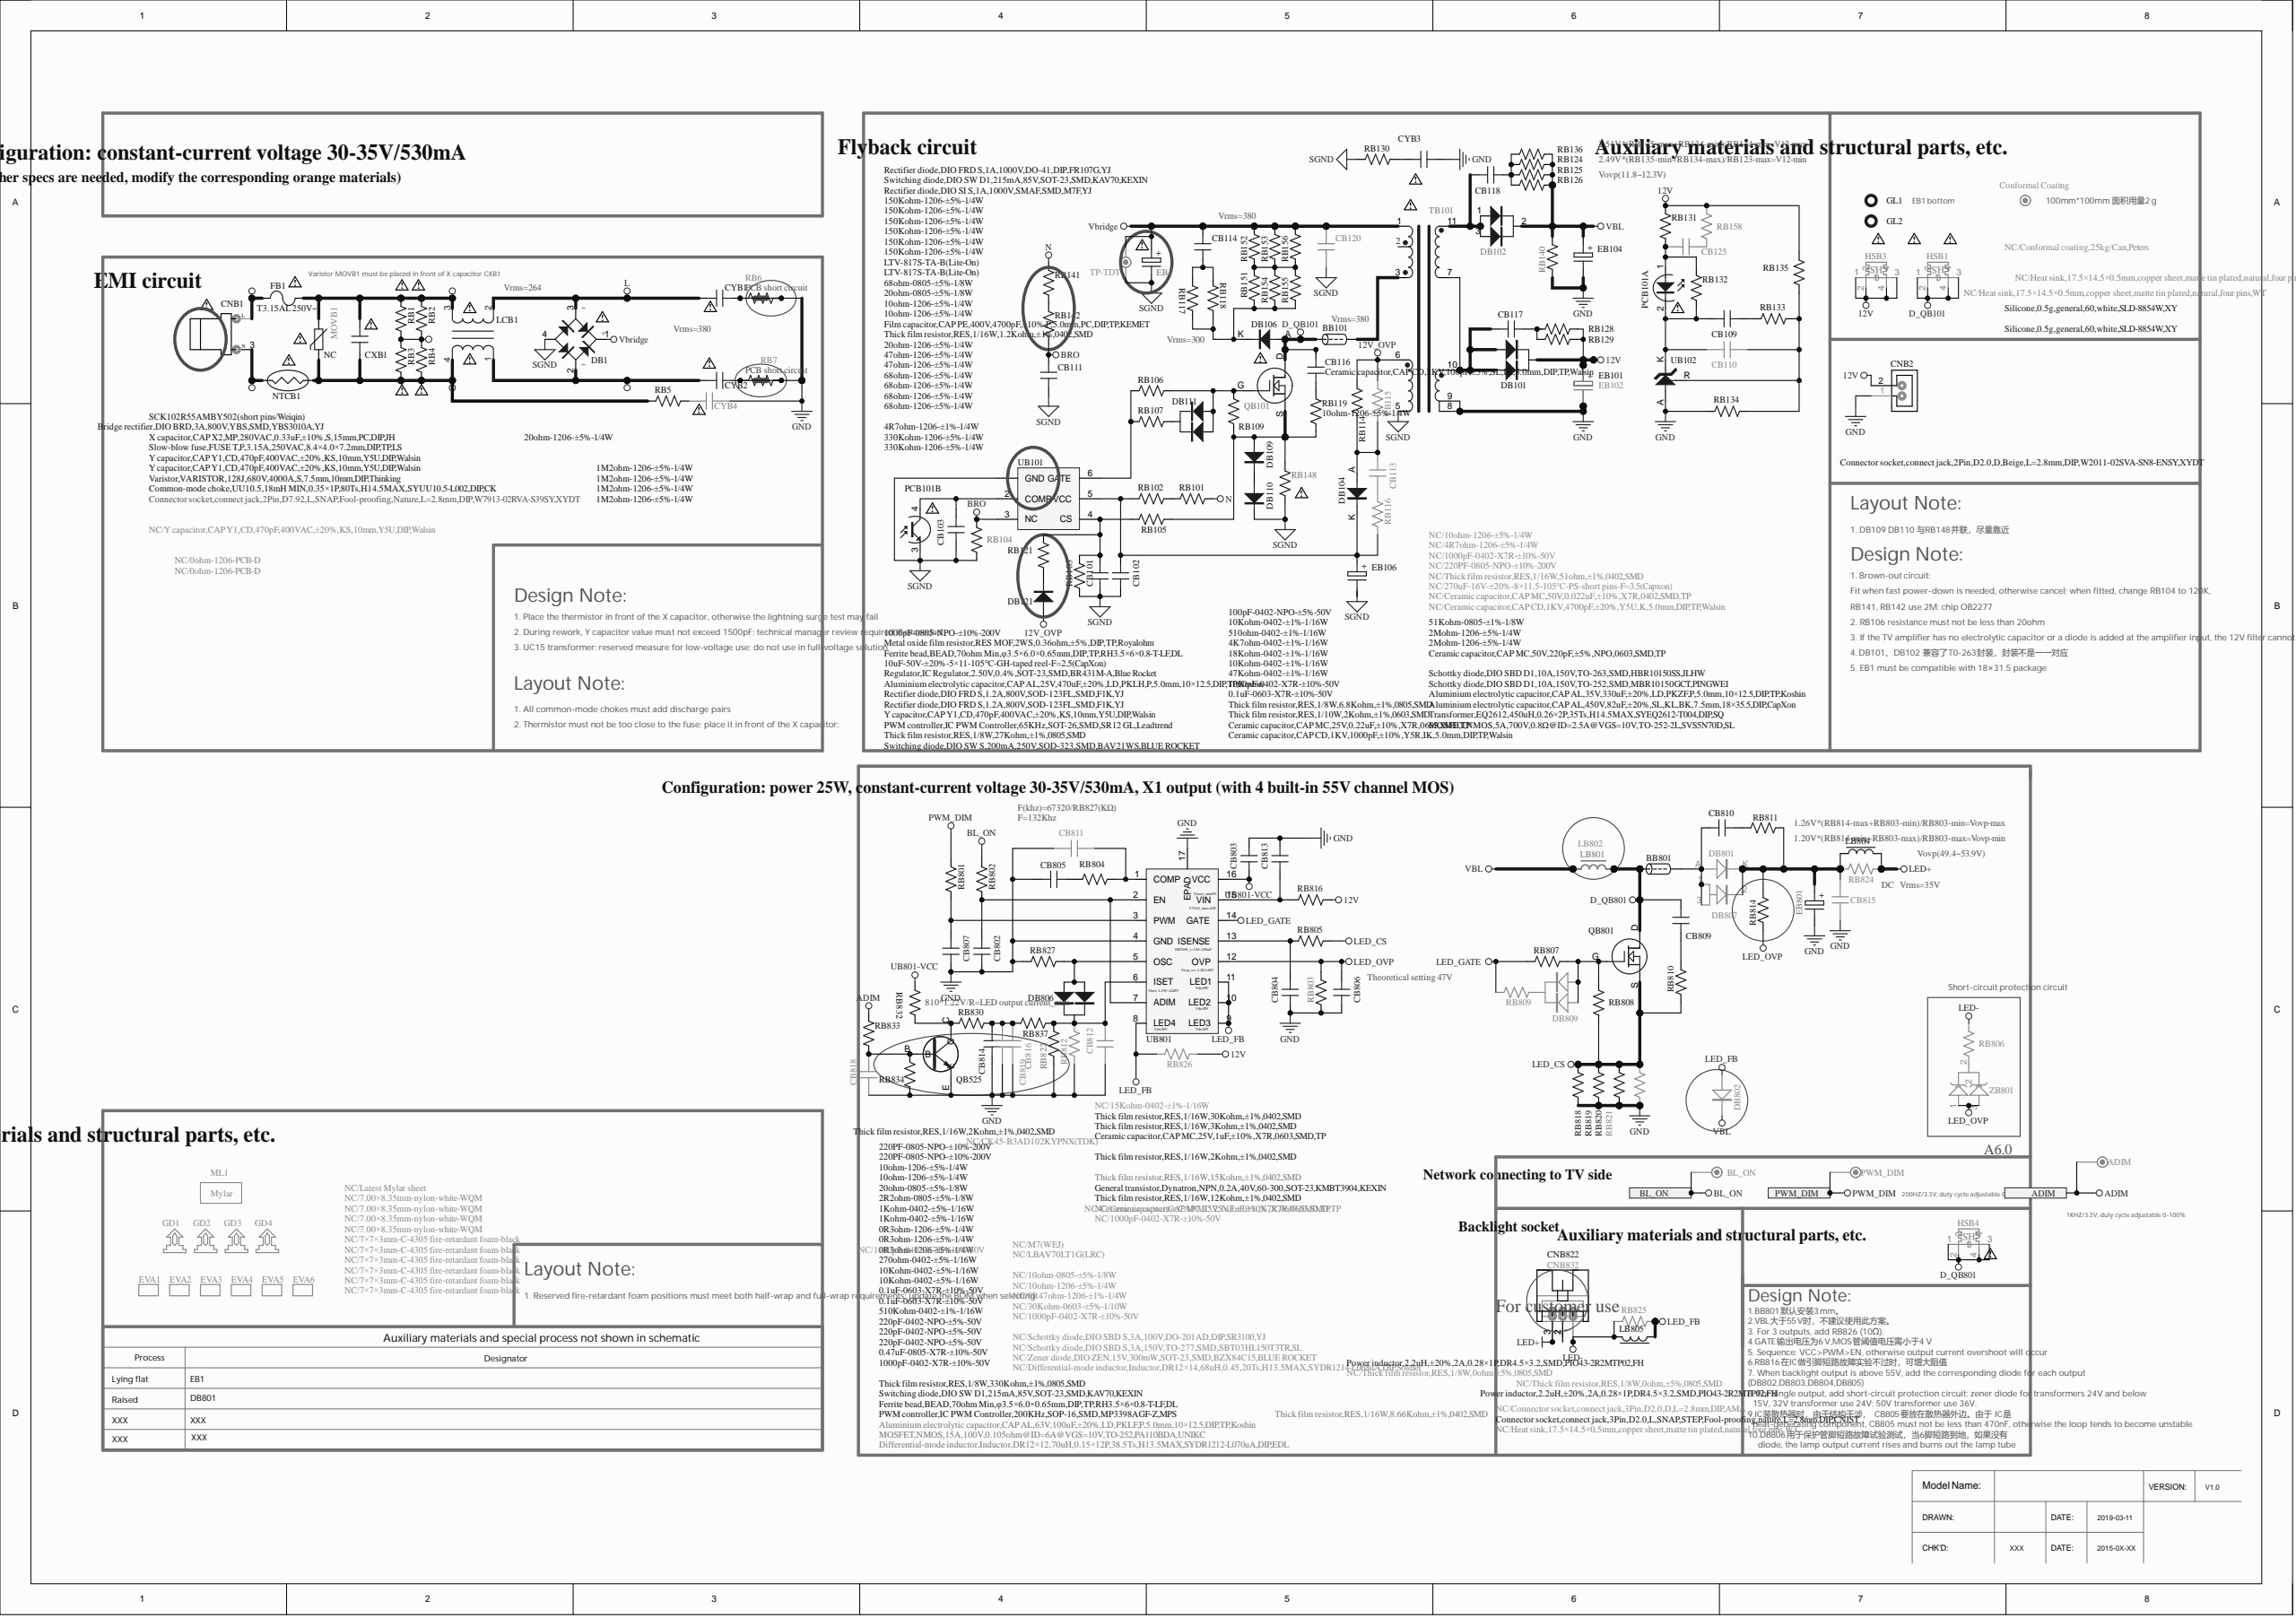Circuit board | Altium Designer | 951 parts | 509 nets | one sheet of the schematic
Parts on this sheet (reference | value | footprint):
BB101 | Ferrite bead,BEAD,70ohm Min,f3.5×6.0×0.65mm,DIP,TP,RH3.5×6×0.8-T-LF,DL | LB/3.5*6*12.5
BB801 | Ferrite bead,BEAD,70ohm Min,f3.5×6.0×0.65mm,DIP,TP,RH3.5×6×0.8-T-LF,DL | LB/3.5*6*12.5
CB101 | 100pF-0402-NPO-±5%-50V | C0402
CB102 | 0.1uF-0603-X7R-±10%-50V | C0603
CB103 | 1000pF-0402-X7R-±10%-50V | C0402
CB109 | Ceramic capacitor,CAP MC,25V,0.22uF,±10%,X7R,0603,SMD,TP | C0603
CB110 | NC/1000pF-0402-X7R-±10%-50V | C0402
CB111 | Ceramic capacitor,CAP MC,50V,220pF,±5%,NPO,0603,SMD,TP | C0603
CB113 | NC/220PF-0805-NPO-±10%-200V | C0805
CB114 | Film capacitor,CAP PE,400V,4700pF,±10%,P,5.0mm,PC,DIP,TP,KEMET | CAP8*2.5-V-5
CB116 | Ceramic capacitor,CAP CD,2KV,100pF,±5%,SL,IK,5.0mm,DIP,TP,Walsin | CAP6.5*5-V-5-1
CB117 | 1000pF-0805-NPO-±10%-200V | C0805
CB118 | Ceramic capacitor,CAP CD,1KV,1000pF,±10%,Y5R,IK,5.0mm,DIP,TP,Walsin | CAP8.5*5-V-5
CB120 | NC/Ceramic capacitor,CAP CD,1KV,4700pF,±20%,Y5U,K,5.0mm,DIP,TP,Walsin | CAP10*4.5-V-5
CB125 | NC/Ceramic capacitor,CAP MC,50V,0.022uF,±10%,X7R,0402,SMD,TP | C0402
CB802 | 220pF-0402-NPO-±5%-50V | C0402
CB803 | 0.1uF-0603-X7R-±10%-50V | C0603
CB804 | 220pF-0402-NPO-±5%-50V | C0402
CB805 | 0.47uF-0805-X7R-±10%-50V | C0805
CB806 | 1000pF-0402-X7R-±10%-50V | C0402
CB807 | 220pF-0402-NPO-±5%-50V | C0402
CB809 | 220PF-0805-NPO-±10%-200V | C0805
CB810 | 220PF-0805-NPO-±10%-200V | C0805
CB811 | NC/1000pF-0402-X7R-±10%-50V | C0402
CB812 | NC/1000pF-0402-X7R-±10%-50V | C0402
CB813 | 0.1uF-0603-X7R-±10%-50V | C0603
CB814 | Ceramic capacitor,CAP MC,25V,1uF,±10%,X7R,0603,SMD,TP | C0603
CB815 | NC/CK45-B3AD102KYPNX(TDK) | CAP7.5*2.5-V-5
CB816 | NC/Ceramic capacitor,CAP MC,25V,1uF,±10%,X7R,0603,SMD,TP | C0603
CB818 | NC/1000pF-0402-X7R-±10%-50V | C0402
CB819 | NC/Ceramic capacitor,CAP MC,25V,1uF,±10%,X7R,0603,SMD,TP | C0603
CNB1 | Connector socket,connect jack,2Pin,D7.92,L,SNAP,Fool-proofing,Nature,L=2.8mm,DIP,W7913-02RVA-S39SY,XYDT | CON2-H7.92
CNB2 | Connector socket,connect jack,2Pin,D2.0,D,Beige,L=2.8mm,DIP,W2011-02SVA-SN8-ENSY,XYDT | SIP2/2.0D-1
CNB822 | Connector socket,connect jack,3Pin,D2.0,L,SNAP,STEP,Fool-proofing,nature,L=2.8mm,DIP,CNJST | SIP3H/2.0D-3
CNB832 | NC/Connector socket,connect jack,3Pin,D2.0,D,L=2.8mm,DIP,AMA | SIP3/2.0D-CP
CXB1 | X capacitor,CAP X2,MP,280VAC,0.33uF,±10%,S,15mm,PC,DIP,JH | CAP18*8.5-V-15
CYB1 | Y capacitor,CAP Y1,CD,470pF,400VAC,±20%,KS,10mm,Y5U,DIP,Walsin | CAP13*5-V-10-1
CYB2 | Y capacitor,CAP Y1,CD,470pF,400VAC,±20%,KS,10mm,Y5U,DIP,Walsin | CAP13*5-V-10-1
CYB3 | Y capacitor,CAP Y1,CD,470pF,400VAC,±20%,KS,10mm,Y5U,DIP,Walsin | CAP13*5-V-10-1
CYB4 | NC/Y capacitor,CAP Y1,CD,470pF,400VAC,±20%,KS,10mm,Y5U,DIP,Walsin | CAP13*5-V-10-1
DB1 | Bridge rectifier,DIO BRD,3A,800V,YBS,SMD,YBS3010A,YJ | B/YBS3010A
DB101 | Schottky diode,DIO SBD D1,10A,150V,TO-252,SMD,MBR10150GCT,PINGWEI | D2PAK3
DB102 | Schottky diode,DIO SBD D1,10A,150V,TO-263,SMD,HBR10150SS,JLHW | D2PAK3
DB104 | Rectifier diode,DIO SI S,1A,1000V,SMAF,SMD,M7F,YJ | DIODE-S-2
DB106 | Rectifier diode,DIO FRD S,1A,1000V,DO-41,DIP,FR107G,YJ | D1-H-17.5
DB109 | Rectifier diode,DIO FRD S,1.2A,800V,SOD-123FL,SMD,F1K,YJ | DIODE-S-14
DB110 | Rectifier diode,DIO FRD S,1.2A,800V,SOD-123FL,SMD,F1K,YJ | DIODE-S-14
DB111 | Switching diode,DIO SW D1,215mA,85V,SOT-23,SMD,KAV70,KEXIN | SO-23
DB121 | Switching diode,DIO SW S,200mA,250V,SOD-323,SMD,BAV21WS,BLUE ROCKET | DIODE-S-12
DB801 | NC/Schottky diode,DIO SBD S,3A,100V,DO-201AD,DIP,SR3100,YJ | D3-H-20
DB802 | NC/M7(WEJ) | DIODE-S-2
DB806 | Switching diode,DIO SW D1,215mA,85V,SOT-23,SMD,KAV70,KEXIN | SO-23
DB807 | NC/Schottky diode,DIO SBD S,3A,150V,TO-277,SMD,SBT03HL150T3TR,SL | DIODE-S-13
DB809 | NC/LBAV70LT1G(LRC) | SO-23
EB1 | Aluminium electrolytic capacitor,CAP AL,450V,82uF,±20%,SL,KL,BK,7.5mm,18×35.5,DIP,CapXon | EC(18*41)-H-7.5-1
EB101 | Aluminium electrolytic capacitor,CAP AL,25V,470uF,±20%,LD,PKLH,P,5.0mm,10×12.5,DIP,TP,Koshin | EC(10*12.5)-V-5
EB102 | NC/270uF-16V-±20%-8×11.5-105℃-PS-short pins-F=3.5(Capxon) | EC(8*11)-V-3.5
EB104 | Aluminium electrolytic capacitor,CAP AL,35V,330uF,±20%,LD,PKZF,P,5.0mm,10×12.5,DIP,TP,Koshin | EC(10*12.5)-V-5
EB106 | 10uF-50V-±20%-5×11-105℃-GH-taped reel-F=2.5(CapXon) | EC(5*11)-V-2.5
EB801 | Aluminium electrolytic capacitor,CAP AL,63V,100uF,±20%,LD,PKLF,P,5.0mm,10×12.5,DIP,TP,Koshin | EC(10*12.5)-V-5
EVA1 | NC/7×7×3mm-C-4305 fire-retardant foam-black | EVA(7*7*3)
EVA2 | NC/7×7×3mm-C-4305 fire-retardant foam-black | EVA(7*7*3)
EVA3 | NC/7×7×3mm-C-4305 fire-retardant foam-black | EVA(7*7*3)
EVA4 | NC/7×7×3mm-C-4305 fire-retardant foam-black | EVA(7*7*3)
EVA5 | NC/7×7×3mm-C-4305 fire-retardant foam-black | EVA(7*7*3)
EVA6 | NC/7×7×3mm-C-4305 fire-retardant foam-black | EVA(7*7*3)
FB1 | Slow-blow fuse,FUSE T,P,3.15A,250VAC,8.4×4.0×7.2mm,DIP,TP,LS | FUSE8.5*4-V-5(T3.15AL 250V~)
GD1 | NC/7.00×8.35mm-nylon-white-WQM | Fixed
GD2 | NC/7.00×8.35mm-nylon-white-WQM | Fixed
GD3 | NC/7.00×8.35mm-nylon-white-WQM | Fixed
GD4 | NC/7.00×8.35mm-nylon-white-WQM | Fixed
GL1 | Silicone,0.5g,general,60,white,SLD-8854W,XY | Silica gel-15
GL2 | Silicone,0.5g,general,60,white,SLD-8854W,XY | Silica gel-10
HSB1 | NC/Heat sink,17.5×14.5×0.5mm,copper sheet,matte tin plated,natural,four pins,WT | HS149-YZ
HSB3 | NC/Heat sink,17.5×14.5×0.5mm,copper sheet,matte tin plated,natural,four pins,WT | HS149-YZ
HSB4 | NC/Heat sink,17.5×14.5×0.5mm,copper sheet,matte tin plated,natural,four pins,WT | HS149-YZ
LB801 | Differential-mode inductor,Inductor,DR12×12,70uH,0.15×12P,38.5Ts,H13.5MAX,SYDR1212-L070uA,DIP,EDL | L/LC2/15*14.5-V7.5
LB802 | NC/Differential-mode inductor,Inductor,DR12×14,68uH,0.45,20Ts,H13.5MAX,SYDR1214-L068uA,DIP,Soldier | L(13.5*15.5)-V-5
LB804 | Power inductor,2.2uH,±20%,2A,0.28×1P,DR4.5×3.2,SMD,PIO43-2R2MTP02,FH | L(4.5*3.5)-S
LB805 | Power inductor,2.2uH,±20%,2A,0.28×1P,DR4.5×3.2,SMD,PIO43-2R2MTP02,FH | L(4.5*3.5)-S
LCB1 | Common-mode choke,UU10.5,18mH MIN,0.35×1P,80Ts,H14.5MAX,SYUU10.5-L002,DIP,CK | L/UU10.5/10*13-2
ML1 | NC/Latest Mylar sheet | Mylar
MOVB1 | Varistor,VARISTOR,128J,680V,4000A,S,7.5mm,10mm,DIP,Thinking | VR(13*5)-V-7.5
NTCB1 | SCK102R55AMBY502(short pins/Weiqin) | NTC(10*5)-V5
PCB101 | LTV-817S-TA-B(Lite-On) | OC4-S-1
QB101 | MOSFET,NMOS,5A,700V,0.8Ω@ID=2.5A@VGS=10V,TO-252-2L,SVS5N70D,SL | TO-252-GDS
QB525 | General transistor,Dynatron,NPN,0.2A,40V,60-300,SOT-23,KMBT3904,KEXIN | SOT-23
QB801 | MOSFET,NMOS,15A,100V,0.105ohm@ID=6A@VGS=10V,TO-252,PA110BDA,UNIKC | TO-252-GDS
RB1 | 1M2ohm-1206-±5%-1/4W | R1206
RB2 | 1M2ohm-1206-±5%-1/4W | R1206
RB3 | 1M2ohm-1206-±5%-1/4W | R1206
RB4 | 1M2ohm-1206-±5%-1/4W | R1206
RB5 | 20ohm-1206-±5%-1/4W | R1206
RB6 | NC/0ohm-1206-PCB-D | R1206SC
RB7 | NC/0ohm-1206-PCB-D | R1206SC
RB101 | 330Kohm-1206-±5%-1/4W | R1206
RB102 | 330Kohm-1206-±5%-1/4W | R1206
RB103 | Thick film resistor,RES,1/8W,6.8Kohm,±1%,0805,SMD | R0402
RB104 | 47Kohm-0402-±1%-1/16W | R0402
RB105 | 510ohm-0402-±1%-1/16W | R0402
RB106 | 68ohm-0805-±5%-1/8W | R0805
RB107 | 20ohm-0805-±5%-1/8W | R0805
RB109 | 10Kohm-0402-±1%-1/16W | R0402
RB114 | 4R7ohm-1206-±1%-1/4W | R1206
RB115 | NC/4R7ohm-1206-±5%-1/4W | R1206
RB116 | NC/10ohm-1206-±5%-1/4W | R1206
RB117 | 10ohm-1206-±5%-1/4W | R1206
RB118 | 10ohm-1206-±5%-1/4W | R1206
RB119 | 10ohm-1206-±5%-1/4W | R1206
RB121 | Thick film resistor,RES,1/8W,27Kohm,±1%,0805,SMD | R0805
RB124 | 68ohm-1206-±5%-1/4W | R1206
RB125 | 68ohm-1206-±5%-1/4W | R1206
RB126 | 68ohm-1206-±5%-1/4W | R1206
RB128 | 47ohm-1206-±5%-1/4W | R1206
RB129 | 47ohm-1206-±5%-1/4W | R1206
RB130 | 20ohm-1206-±5%-1/4W | R1206
RB131 | Thick film resistor,RES,1/10W,2Kohm,±1%,0603,SMD | R0603
RB132 | Thick film resistor,RES,1/16W,1.2Kohm,±1%,0402,SMD | R0402
RB133 | 10Kohm-0402-±1%-1/16W | R0402
RB134 | 4K7ohm-0402-±1%-1/16W | R0402
RB135 | 18Kohm-0402-±1%-1/16W | R0402
RB136 | 68ohm-1206-±5%-1/4W | R1206
RB140 | 51Kohm-0805-±1%-1/8W | R0805
RB141 | 2Mohm-1206-±5%-1/4W | R1206
RB142 | 2Mohm-1206-±5%-1/4W | R1206
RB148 | Metal oxide film resistor,RES MOF,2WS,0.36ohm,±5%,DIP,TP,Royalohm | R2-H-17.5
RB151 | 150Kohm-1206-±5%-1/4W | R1206
RB152 | 150Kohm-1206-±5%-1/4W | R1206
RB153 | 150Kohm-1206-±5%-1/4W | R1206
RB154 | 150Kohm-1206-±5%-1/4W | R1206
RB155 | 150Kohm-1206-±5%-1/4W | R1206
RB156 | 150Kohm-1206-±5%-1/4W | R1206
RB158 | NC/Thick film resistor,RES,1/16W,51ohm,±1%,0402,SMD | R0402
RB801 | 1Kohm-0402-±5%-1/16W | R0402
RB802 | 10Kohm-0402-±5%-1/16W | R0402
RB803 | Thick film resistor,RES,1/16W,8.66Kohm,±1%,0402,SMD | R0402
RB804 | 270ohm-0402-±5%-1/16W | R0402
RB805 | 1Kohm-0402-±5%-1/16W | R0402
RB806 | NC/30Kohm-0603-±5%-1/10W | R0603
RB807 | 20ohm-0805-±5%-1/8W | R0805
RB808 | 10Kohm-0402-±5%-1/16W | R0402
RB809 | NC/10ohm-0805-±5%-1/8W | R0805
RB810 | 10ohm-1206-±5%-1/4W | R1206
RB811 | 10ohm-1206-±5%-1/4W | R1206
RB812 | NC/15Kohm-0402-±1%-1/16W | R0402
RB814 | Thick film resistor,RES,1/8W,330Kohm,±1%,0805,SMD | R0805
RB816 | 2R2ohm-0805-±5%-1/8W | R0805
RB818 | 0R3ohm-1206-±5%-1/4W | R1206
RB819 | 0R3ohm-1206-±5%-1/4W | R1206
RB820 | 0R3ohm-1206-±5%-1/4W | R1206
RB821 | NC/0R47ohm-1206-±1%-1/4W | R1206
RB822 | Thick film resistor,RES,1/16W,15Kohm,±1%,0402,SMD | R0402
RB824 | NC/Thick film resistor,RES,1/8W,0ohm,±5%,0805,SMD | R0805
RB825 | NC/Thick film resistor,RES,1/8W,0ohm,±5%,0805,SMD | R0805
RB826 | NC/10ohm-1206-±5%-1/4W | R1206
RB827 | 510Kohm-0402-±1%-1/16W | R0402
RB830 | Thick film resistor,RES,1/16W,3Kohm,±1%,0402,SMD | R0402
RB832 | Thick film resistor,RES,1/16W,30Kohm,±1%,0402,SMD | R0402
RB833 | Thick film resistor,RES,1/16W,2Kohm,±1%,0402,SMD | R0402
RB834 | Thick film resistor,RES,1/16W,2Kohm,±1%,0402,SMD | R0402
RB837 | Thick film resistor,RES,1/16W,12Kohm,±1%,0402,SMD | R0402
TB101 | Transformer,EQ2612,450uH,0.26×2P,35Ts,H14.5MAX,SYEQ2612-T004,DIP,SQ | T/EQ2512*11
TP-TDT | NC/ | TP-TDT
UB101 | PWM controller,IC PWM Controller,65KHz,SOT-26,SMD,SR12 GL,Leadtrend | SOT-26
UB102 | Regulator,IC Regulator,2.50V,0.4%,SOT-23,SMD,BR431M-A,Blue Rocket | SOT-23-RAK
UB801 | PWM controller,IC PWM Controller,200KHz,SOP-16,SMD,MP3398AGF-Z,MPS | TSSOP16/0.65-3
ZB801 | NC/Zener diode,DIO ZEN,15V,300mW,SOT-23,SMD,BZX84C15,BLUE ROCKET | SO-23
Nets of these parts (net: part-pin ...):
Vbridge: CB114-2 CB120-2 DB1-1 EB1-1 RB152-2 RB153-2 RB156-2 TB101-1 TP-TDT-1
VBL: DB102-2 DB802-K EB104-1 LB801-1 LB802-1 RB124-2 RB125-2 RB126-2 RB136-2 RB140-1
UB801-VCC: CB803-2 RB832-1 UB801-16
SGND: CB101-2 CB102-2 CB103-2 CB111-1 CB120-1 DB1-4 DB110-K EB1-2 EB106-2 PCB101-3 RB103-1 RB104-1 RB130-1 RB148-1 TB101-5 TP-TDT-2 UB101-1
PWM_DIM: RB801-1
NetRB806_2: RB806-2 ZB801-2
NetRB151_2: RB151-2 RB152-1 RB153-1 RB154-2 RB155-2 RB156-1
NetRB141_1: RB141-1 RB142-2
NetRB106_1: RB106-1 RB107-1 UB101-6
NetRB101_2: RB101-2 RB102-2
NetQB525_C: QB525-C RB830-2 RB832-2
NetDB809_2: DB809-2 RB809-2
NetDB809_1: DB809-1 DB809-3 QB801-G RB807-2 RB808-1
NetDB806_1: DB806-1 DB806-3 RB827-2 UB801-5
NetDB121_K: DB121-K RB121-1
NetDB111_2: DB111-2 RB107-2
NetDB111_1: DB111-1 DB111-3 QB101-G RB106-2 RB109-2
NetDB109_K: DB109-K DB110-A
NetDB109_A: DB109-A QB101-S RB105-2 RB109-1 RB119-1 RB148-2
NetDB106_K: DB106-K RB117-2 RB118-2 RB151-1 RB154-1 RB155-1
NetCYB4_1: CYB4-1 RB5-1
NetCYB3_1: CYB3-1 RB130-2
NetCNB822_2: CNB822-2 CNB832-2
NetCB818_2: CB818-2 QB525-B RB833-1 RB834-2
NetCB815_1: CB815-1 DB801-K DB807-2 EB801-1 LB804-1 RB811-2 RB814-2 RB824-1
NetCB814_1: CB814-1 CB816-1 CB819-1 RB830-1 RB837-1
NetCB813_2: CB813-2 RB816-1 UB801-15
NetCB812_2: CB812-2 DB806-2 RB812-2 RB822-2 RB837-2 UB801-6
NetCB811_1: CB811-1 RB804-2 UB801-1
NetCB810_1: CB810-1 RB811-1
NetCB809_1: CB809-1 RB810-1
NetCB807_1: CB807-1 RB801-2 UB801-3
NetCB805_2: CB805-2 RB804-1
NetCB804_2: CB804-2 RB805-2 UB801-13
NetCB802_2: CB802-2 RB802-2 UB801-2 UB801-7
NetCB125_2: CB125-2 RB158-1
NetCB125_1: CB125-1 PCB101-1 RB131-1 RB132-2
NetCB118_2: CB118-2 RB124-1 RB125-1 RB126-1 RB136-1
NetCB118_1: CB118-1 DB102-1 DB102-3 TB101-11
NetCB117_2: CB117-2 RB128-1 RB129-1
NetCB117_1: CB117-1 DB101-1 DB101-3 TB101-7 TB101-10
NetCB116_1: CB116-1 RB119-2
NetCB114_1: CB114-1 RB117-1 RB118-1
NetCB113_2: CB113-2 RB116-2
NetCB113_1: CB113-1 DB104-A RB114-1 RB115-1
NetCB110_2: CB110-2 RB133-2 RB134-2 RB135-2 UB102-R
NetCB109_2: CB109-2 RB133-1
NetCB109_1: CB109-1 CB110-1 PCB101-2 RB132-1 UB102-K
NetCB103_1: CB103-1 PCB101-4 UB101-2
NetCB102_1: CB102-1 DB104-K EB106-1 RB102-1 RB116-1 UB101-5
NetCB101_1: CB101-1 RB103-2 RB105-1 RB121-2 UB101-4
NetBB801_2: BB801-2 CB810-2 DB801-A DB807-1 DB807-3
NetBB101_2: BB101-2 TB101-3
N-2: CXB1-2 LCB1-4 MOVB1-2 NTCB1-1 RB3-2 RB4-2 RB5-2
N-1: CNB1-3 NTCB1-2
N: CYB2-1 DB1-2 LCB1-1 RB101-1 RB141-2
LED_OVP: CB806-2 RB803-2 RB814-1 UB801-12 ZB801-1 ZB801-3
LED_GATE: RB807-1 RB809-1 UB801-14
LED_FB: DB802-A LB805-2 RB825-1 RB826-1 UB801-8 UB801-9 UB801-10 UB801-11
LED_CS: QB801-S RB805-1 RB808-2 RB810-2 RB818-1 RB819-1 RB820-1 RB821-1
LED-: CNB822-1 CNB832-1 LB805-1 RB806-1 RB825-2
LED+: CNB822-3 CNB832-3 LB804-2 RB824-2
L-N: RB1-2 RB2-2 RB3-1 RB4-1
L-2: CXB1-1 FB1-2 LCB1-3 MOVB1-1 RB1-1 RB2-1
L-1: CNB1-1 FB1-1
L: CYB1-1 DB1-3 LCB1-2
GND: CB802-1 CB803-1 CB804-1 CB805-1 CB806-1 CB807-2 CB811-2 CB812-1 CB813-1 CB814-2 CB815-2 CB816-2 CB818-1 CB819-2 CNB2-1 CYB1-2 CYB2-2 CYB3-2 CYB4-2 EB101-2 EB102-2 EB104-2 EB801-2 QB525-E RB6-1 RB6-2 RB6-3 RB7-1 RB7-2 RB7-3 RB134-1 RB140-2 RB803-1 RB812-1 RB818-2 RB819-2 RB820-2 RB821-2 RB822-1 RB827-1 RB834-1 TB101-8 TB101-9 UB102-A UB801-4 UB801-17
D_QB801: BB801-1 CB809-2 HSB4-1 HSB4-2 HSB4-3 HSB4-4 LB801-2 LB802-2 QB801-D
D_QB101: BB101-1 CB116-2 DB106-A HSB1-1 HSB1-2 HSB1-3 HSB1-4 QB101-D
BRO: CB111-2 RB104-2 RB142-1 UB101-3
BL_ON: RB802-1
ADIM: RB833-2
12V_OVP: DB121-A RB114-2 RB115-2 TB101-6
12V: CNB2-2 DB101-2 EB101-1 EB102-1 HSB3-1 HSB3-2 HSB3-3 HSB3-4 RB128-2 RB129-2 RB131-2 RB135-1 RB158-2 RB816-2 RB826-2